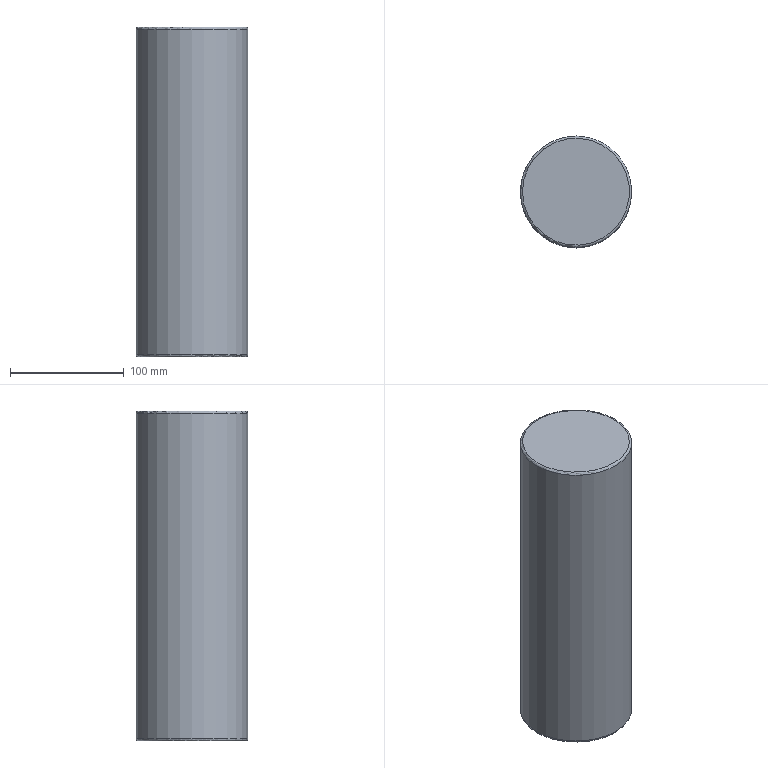Part | STEP file | solid 2 | 1 solid | 19 faces | box 98 x 98 x 290 mm | volume 2182712 mm3 | plane 11 | cylinder 2 | torus 2 | other 2 | cone 2 | commonest cylinder face diameters 14 x1 98 x1